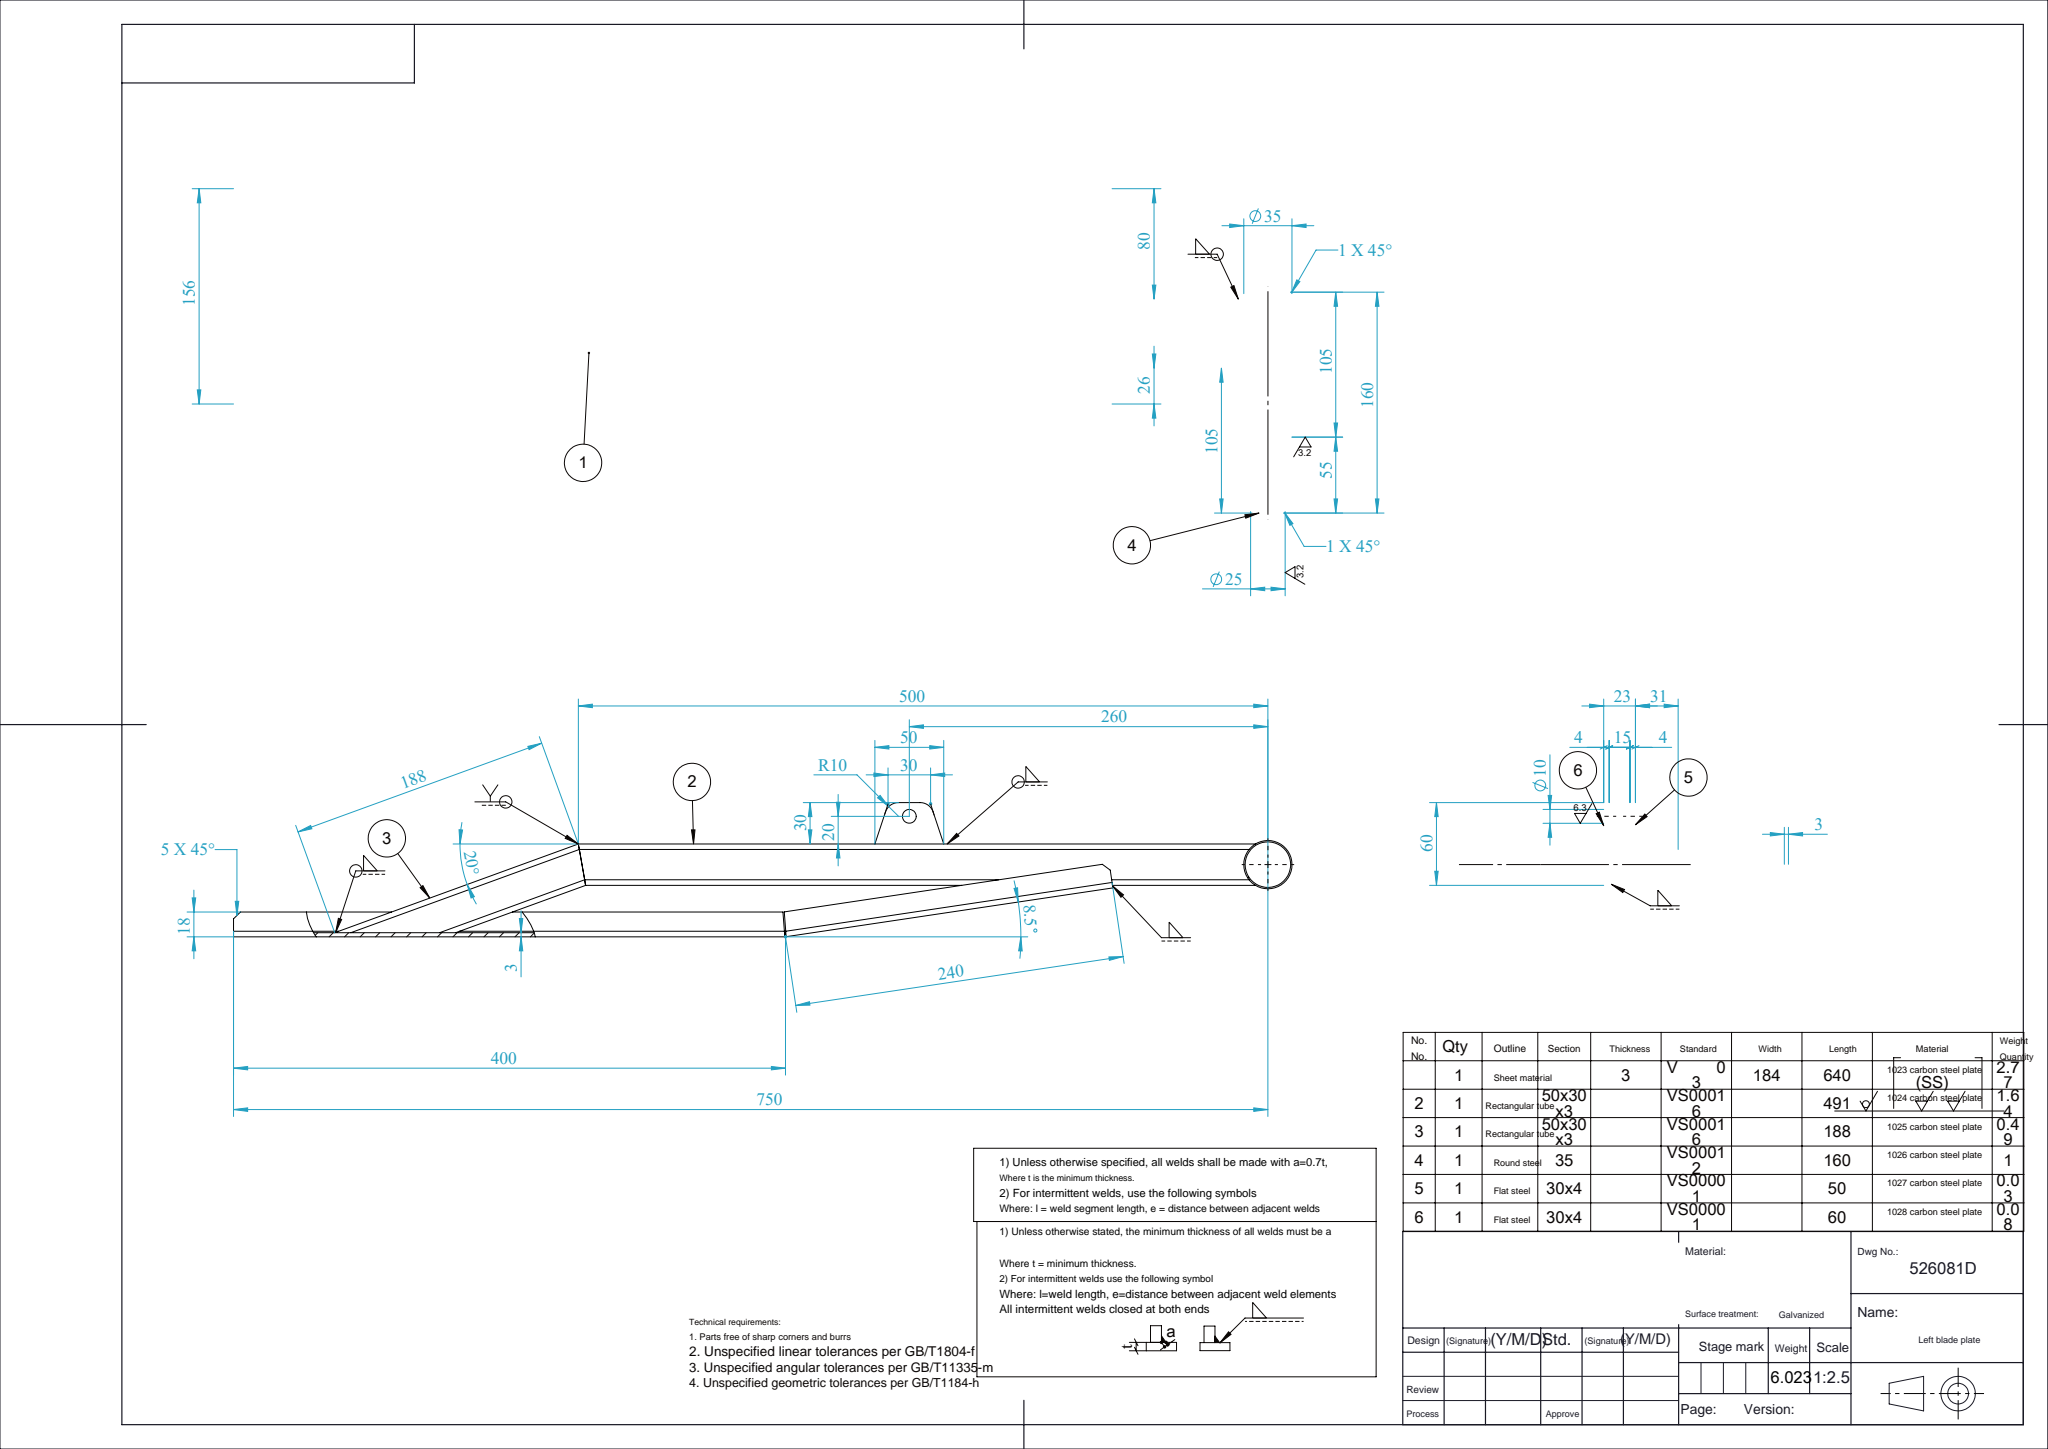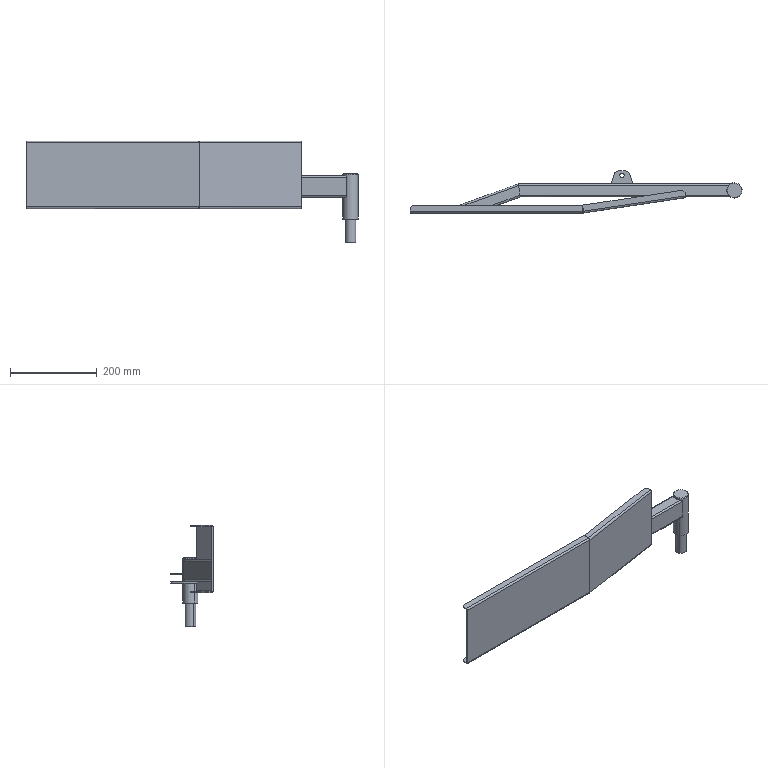Part | SolidWorks | features CompositeCurve 7 | 6 solids | 123 faces | box 767.5 x 97.3 x 235 mm | volume 766450 mm3 | plane 76 | cylinder 39 | spline 4 | cone 4 | commonest cylinder face diameters 2 x12 8 x12 10 x4 20 x4 35 x3 25 x2